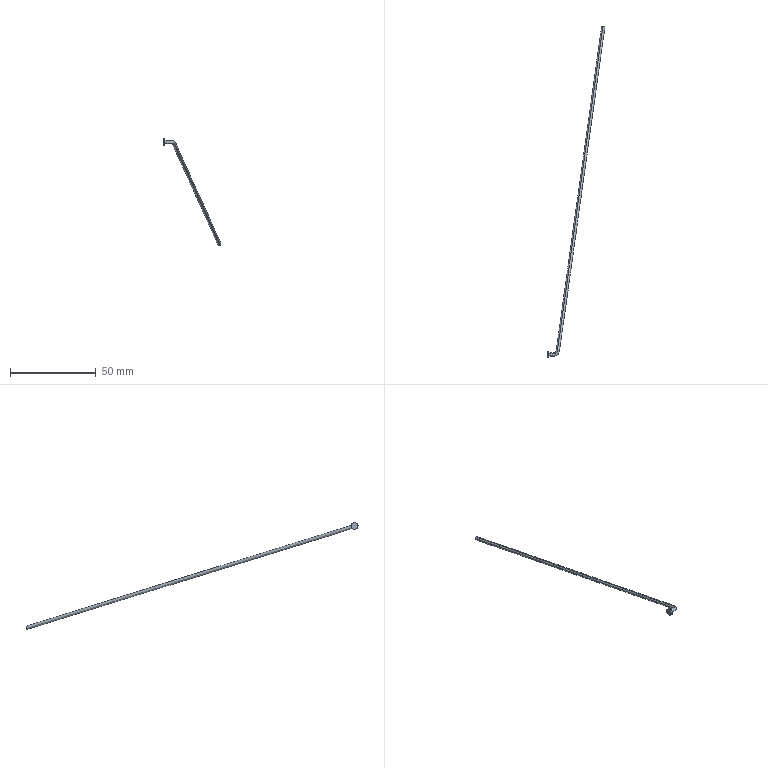Part | STEP file | BREP_52 | 1 solid | 7 faces | box 33.776 x 193.437 x 62.153 mm | volume 645.284 mm3 | plane 3 | cylinder 2 | spline 2 | commonest cylinder face diameters 4 x2